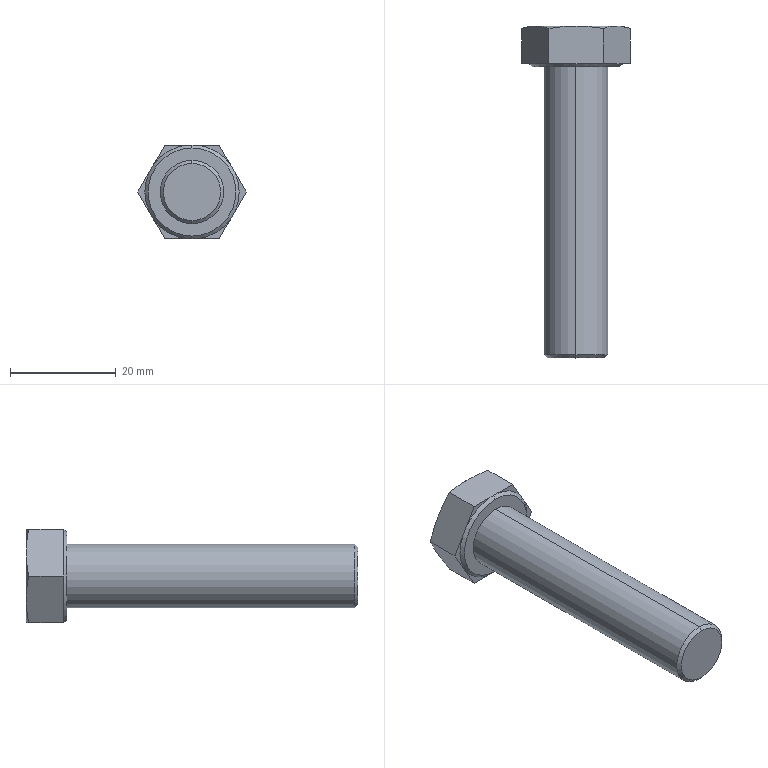Part | NX | features BREP 1 | 1 solid | 27 faces | box 20.473 x 62.68 x 17.73 mm | volume 8277 mm3 | plane 15 | cone 10 | cylinder 2 | commonest cylinder face diameters 12 x2
STEP:
#1=CARTESIAN_POINT('',(-41.42,-20.14,45.6));
#2=VERTEX_POINT('',#1);
#3=CARTESIAN_POINT('',(-41.42,-20.14,56.4));
#4=VERTEX_POINT('',#3);
#5=CARTESIAN_POINT('',(-41.42,-20.14,51.));
#6=DIRECTION('',(0.,-1.,0.));
#7=DIRECTION('',(0.,0.,-1.));
#8=AXIS2_PLACEMENT_3D('',#5,#6,#7);
#9=CIRCLE('',#8,5.4);
#10=EDGE_CURVE('',#2,#4,#9,.T.);
#11=ORIENTED_EDGE('',*,*,#10,.F.);
#12=CARTESIAN_POINT('',(-41.42,-19.54,45.));
#13=VERTEX_POINT('',#12);
#14=CARTESIAN_POINT('',(-41.42,-20.14,45.6));
#15=DIRECTION('',(0.,0.7071,-0.7071));
#16=VECTOR('',#15,1000.);
#17=LINE('',#14,#16);
#18=EDGE_CURVE('',#2,#13,#17,.T.);
#19=ORIENTED_EDGE('',*,*,#18,.T.);
#20=CARTESIAN_POINT('',(-41.42,-19.54,57.));
#21=VERTEX_POINT('',#20);
#22=CARTESIAN_POINT('',(-41.42,-19.54,51.));
#23=DIRECTION('',(0.,1.,0.));
#24=DIRECTION('',(0.,0.,-1.));
#25=AXIS2_PLACEMENT_3D('',#22,#23,#24);
#26=CIRCLE('',#25,6.);
#27=EDGE_CURVE('',#21,#13,#26,.T.);
#28=ORIENTED_EDGE('',*,*,#27,.F.);
#29=CARTESIAN_POINT('',(-41.42,-20.14,56.4));
#30=DIRECTION('',(0.,0.7071,0.7071));
#31=VECTOR('',#30,1000.);
#32=LINE('',#29,#31);
#33=EDGE_CURVE('',#4,#21,#32,.T.);
#34=ORIENTED_EDGE('',*,*,#33,.F.);
#35=EDGE_LOOP('',(#11,#19,#28,#34));
#36=FACE_BOUND('',#35,.T.);
#37=CARTESIAN_POINT('',(-41.42,-20.14,51.));
#38=DIRECTION('',(0.,1.,0.));
#39=DIRECTION('',(0.,0.,-1.));
#40=AXIS2_PLACEMENT_3D('',#37,#38,#39);
#41=CONICAL_SURFACE('',#40,5.4,0.7854);
#42=ADVANCED_FACE('',(#36),#41,.T.);
#43=ORIENTED_EDGE('',*,*,#27,.T.);
#44=CARTESIAN_POINT('',(-41.42,34.86,45.));
#45=VERTEX_POINT('',#44);
#46=CARTESIAN_POINT('',(-41.42,-20.14,45.));
#47=DIRECTION('',(0.,1.,0.));
#48=VECTOR('',#47,1000.);
#49=LINE('',#46,#48);
#50=EDGE_CURVE('',#13,#45,#49,.T.);
#51=ORIENTED_EDGE('',*,*,#50,.T.);
#52=CARTESIAN_POINT('',(-41.42,34.86,57.));
#53=VERTEX_POINT('',#52);
#54=CARTESIAN_POINT('',(-41.42,34.86,51.));
#55=DIRECTION('',(0.,-1.,0.));
#56=DIRECTION('',(0.,0.,-1.));
#57=AXIS2_PLACEMENT_3D('',#54,#55,#56);
#58=CIRCLE('',#57,6.);
#59=EDGE_CURVE('',#45,#53,#58,.T.);
#60=ORIENTED_EDGE('',*,*,#59,.T.);
#61=CARTESIAN_POINT('',(-41.42,-20.14,57.));
#62=DIRECTION('',(0.,1.,0.));
#63=VECTOR('',#62,1000.);
#64=LINE('',#61,#63);
#65=EDGE_CURVE('',#21,#53,#64,.T.);
#66=ORIENTED_EDGE('',*,*,#65,.F.);
#67=EDGE_LOOP('',(#43,#51,#60,#66));
#68=FACE_BOUND('',#67,.T.);
#69=CARTESIAN_POINT('',(-41.42,-20.14,51.));
#70=DIRECTION('',(0.,1.,0.));
#71=DIRECTION('',(0.,0.,-1.));
#72=AXIS2_PLACEMENT_3D('',#69,#70,#71);
#73=CYLINDRICAL_SURFACE('',#72,6.);
#74=ADVANCED_FACE('',(#68),#73,.T.);
#75=CARTESIAN_POINT('',(-41.42,34.86,59.315));
#76=VERTEX_POINT('',#75);
#77=CARTESIAN_POINT('',(-41.42,34.86,42.685));
#78=VERTEX_POINT('',#77);
#79=CARTESIAN_POINT('',(-41.42,34.86,51.));
#80=DIRECTION('',(0.,1.,0.));
#81=DIRECTION('',(0.,0.,1.));
#82=AXIS2_PLACEMENT_3D('',#79,#80,#81);
#83=CIRCLE('',#82,8.315);
#84=EDGE_CURVE('',#76,#78,#83,.T.);
#85=ORIENTED_EDGE('',*,*,#84,.T.);
#86=CARTESIAN_POINT('',(-41.42,35.41,42.135));
#87=VERTEX_POINT('',#86);
#88=CARTESIAN_POINT('',(-41.42,35.46,42.085));
#89=DIRECTION('',(0.,0.7071,-0.7071));
#90=VECTOR('',#89,1000.);
#91=LINE('',#88,#90);
#92=EDGE_CURVE('',#78,#87,#91,.T.);
#93=ORIENTED_EDGE('',*,*,#92,.T.);
#94=CARTESIAN_POINT('',(-40.477,35.46,42.135));
#95=VERTEX_POINT('',#94);
#96=CARTESIAN_POINT('',(-41.42,35.41,42.135));
#97=CARTESIAN_POINT('',(-41.106,35.41,42.135));
#98=CARTESIAN_POINT('',(-40.791,35.427,42.135));
#99=CARTESIAN_POINT('',(-40.477,35.46,42.135));
#100=B_SPLINE_CURVE_WITH_KNOTS('',3,(#96,#97,#98,#99),.UNSPECIFIED.,.F.,.F.,(4,4),(0.,1.),.PIECEWISE_BEZIER_KNOTS.);
#101=EDGE_CURVE('',#87,#95,#100,.T.);
#102=ORIENTED_EDGE('',*,*,#101,.T.);
#103=CARTESIAN_POINT('',(-34.214,35.46,45.751));
#104=VERTEX_POINT('',#103);
#105=CARTESIAN_POINT('',(-41.42,35.46,51.));
#106=DIRECTION('',(0.,1.,0.));
#107=DIRECTION('',(0.,0.,1.));
#108=AXIS2_PLACEMENT_3D('',#105,#106,#107);
#109=CIRCLE('',#108,8.915);
#110=EDGE_CURVE('',#104,#95,#109,.T.);
#111=ORIENTED_EDGE('',*,*,#110,.F.);
#112=CARTESIAN_POINT('',(-33.271,35.46,47.384));
#113=VERTEX_POINT('',#112);
#114=CARTESIAN_POINT('',(-34.214,35.46,45.751));
#115=CARTESIAN_POINT('',(-33.9,35.394,46.295));
#116=CARTESIAN_POINT('',(-33.586,35.394,46.84));
#117=CARTESIAN_POINT('',(-33.271,35.46,47.384));
#118=B_SPLINE_CURVE_WITH_KNOTS('',3,(#114,#115,#116,#117),.UNSPECIFIED.,.F.,.F.,(4,4),(0.,0.001886),.UNSPECIFIED.);
#119=EDGE_CURVE('',#104,#113,#118,.T.);
#120=ORIENTED_EDGE('',*,*,#119,.T.);
#121=CARTESIAN_POINT('',(-33.271,35.46,54.616));
#122=VERTEX_POINT('',#121);
#123=CARTESIAN_POINT('',(-41.42,35.46,51.));
#124=DIRECTION('',(0.,1.,0.));
#125=DIRECTION('',(0.,0.,1.));
#126=AXIS2_PLACEMENT_3D('',#123,#124,#125);
#127=CIRCLE('',#126,8.915);
#128=EDGE_CURVE('',#122,#113,#127,.T.);
#129=ORIENTED_EDGE('',*,*,#128,.F.);
#130=CARTESIAN_POINT('',(-34.214,35.46,56.249));
#131=VERTEX_POINT('',#130);
#132=CARTESIAN_POINT('',(-33.271,35.46,54.616));
#133=CARTESIAN_POINT('',(-33.586,35.394,55.16));
#134=CARTESIAN_POINT('',(-33.9,35.394,55.705));
#135=CARTESIAN_POINT('',(-34.214,35.46,56.249));
#136=B_SPLINE_CURVE_WITH_KNOTS('',3,(#132,#133,#134,#135),.UNSPECIFIED.,.F.,.F.,(4,4),(0.,0.001886),.UNSPECIFIED.);
#137=EDGE_CURVE('',#122,#131,#136,.T.);
#138=ORIENTED_EDGE('',*,*,#137,.T.);
#139=CARTESIAN_POINT('',(-40.477,35.46,59.865));
#140=VERTEX_POINT('',#139);
#141=CARTESIAN_POINT('',(-41.42,35.46,51.));
#142=DIRECTION('',(0.,1.,0.));
#143=DIRECTION('',(0.,0.,1.));
#144=AXIS2_PLACEMENT_3D('',#141,#142,#143);
#145=CIRCLE('',#144,8.915);
#146=EDGE_CURVE('',#140,#131,#145,.T.);
#147=ORIENTED_EDGE('',*,*,#146,.F.);
#148=CARTESIAN_POINT('',(-41.42,35.41,59.865));
#149=VERTEX_POINT('',#148);
#150=CARTESIAN_POINT('',(-40.477,35.46,59.865));
#151=CARTESIAN_POINT('',(-40.791,35.427,59.865));
#152=CARTESIAN_POINT('',(-41.106,35.41,59.865));
#153=CARTESIAN_POINT('',(-41.42,35.41,59.865));
#154=B_SPLINE_CURVE_WITH_KNOTS('',3,(#150,#151,#152,#153),.UNSPECIFIED.,.F.,.F.,(4,4),(0.,1.),.PIECEWISE_BEZIER_KNOTS.);
#155=EDGE_CURVE('',#140,#149,#154,.T.);
#156=ORIENTED_EDGE('',*,*,#155,.T.);
#157=CARTESIAN_POINT('',(-41.42,35.46,59.915));
#158=DIRECTION('',(0.,0.7071,0.7071));
#159=VECTOR('',#158,1000.);
#160=LINE('',#157,#159);
#161=EDGE_CURVE('',#76,#149,#160,.T.);
#162=ORIENTED_EDGE('',*,*,#161,.F.);
#163=EDGE_LOOP('',(#85,#93,#102,#111,#120,#129,#138,#147,#156,#162));
#164=FACE_BOUND('',#163,.T.);
#165=CARTESIAN_POINT('',(-41.42,35.46,51.));
#166=DIRECTION('',(0.,1.,0.));
#167=DIRECTION('',(0.,0.,-1.));
#168=AXIS2_PLACEMENT_3D('',#165,#166,#167);
#169=CONICAL_SURFACE('',#168,8.915,0.7854);
#170=ADVANCED_FACE('',(#164),#169,.T.);
#171=ORIENTED_EDGE('',*,*,#84,.F.);
#172=CARTESIAN_POINT('',(-41.42,34.86,51.));
#173=DIRECTION('',(0.,1.,0.));
#174=DIRECTION('',(0.,0.,1.));
#175=AXIS2_PLACEMENT_3D('',#172,#173,#174);
#176=CIRCLE('',#175,8.315);
#177=EDGE_CURVE('',#78,#76,#176,.T.);
#178=ORIENTED_EDGE('',*,*,#177,.F.);
#179=EDGE_LOOP('',(#171,#178));
#180=FACE_BOUND('',#179,.T.);
#181=CARTESIAN_POINT('',(-41.42,34.86,51.));
#182=DIRECTION('',(0.,-1.,0.));
#183=DIRECTION('',(0.,0.,-1.));
#184=AXIS2_PLACEMENT_3D('',#181,#182,#183);
#185=CIRCLE('',#184,6.);
#186=EDGE_CURVE('',#53,#45,#185,.T.);
#187=ORIENTED_EDGE('',*,*,#186,.F.);
#188=ORIENTED_EDGE('',*,*,#59,.F.);
#189=EDGE_LOOP('',(#187,#188));
#190=FACE_BOUND('',#189,.T.);
#191=CARTESIAN_POINT('',(-46.538,34.86,42.135));
#192=DIRECTION('',(0.,-1.,0.));
#193=DIRECTION('',(0.,0.,1.));
#194=AXIS2_PLACEMENT_3D('',#191,#192,#193);
#195=PLANE('',#194);
#196=ADVANCED_FACE('',(#180,#190),#195,.T.);
#197=CARTESIAN_POINT('',(-46.538,42.041,42.135));
#198=VERTEX_POINT('',#197);
#199=CARTESIAN_POINT('',(-49.097,42.54,46.568));
#200=VERTEX_POINT('',#199);
#201=CARTESIAN_POINT('',(-46.538,42.041,42.135));
#202=CARTESIAN_POINT('',(-47.384,42.349,43.601));
#203=CARTESIAN_POINT('',(-48.236,42.54,45.076));
#204=CARTESIAN_POINT('',(-49.097,42.54,46.568));
#205=B_SPLINE_CURVE_WITH_KNOTS('',3,(#201,#202,#203,#204),.UNSPECIFIED.,.F.,.F.,(4,4),(0.,0.005142),.UNSPECIFIED.);
#206=EDGE_CURVE('',#198,#200,#205,.T.);
#207=ORIENTED_EDGE('',*,*,#206,.F.);
#208=CARTESIAN_POINT('',(-46.538,35.46,42.135));
#209=VERTEX_POINT('',#208);
#210=CARTESIAN_POINT('',(-46.538,34.86,42.135));
#211=DIRECTION('',(0.,1.,0.));
#212=VECTOR('',#211,1000.);
#213=LINE('',#210,#212);
#214=EDGE_CURVE('',#209,#198,#213,.T.);
#215=ORIENTED_EDGE('',*,*,#214,.F.);
#216=CARTESIAN_POINT('',(-48.626,35.46,45.751));
#217=VERTEX_POINT('',#216);
#218=CARTESIAN_POINT('',(-51.656,35.46,51.));
#219=DIRECTION('',(0.5,0.,-0.866));
#220=VECTOR('',#219,1000.);
#221=LINE('',#218,#220);
#222=EDGE_CURVE('',#217,#209,#221,.T.);
#223=ORIENTED_EDGE('',*,*,#222,.F.);
#224=CARTESIAN_POINT('',(-49.569,35.46,47.384));
#225=VERTEX_POINT('',#224);
#226=CARTESIAN_POINT('',(-49.569,35.46,47.384));
#227=CARTESIAN_POINT('',(-49.255,35.394,46.84));
#228=CARTESIAN_POINT('',(-48.94,35.394,46.295));
#229=CARTESIAN_POINT('',(-48.626,35.46,45.751));
#230=B_SPLINE_CURVE_WITH_KNOTS('',3,(#226,#227,#228,#229),.UNSPECIFIED.,.F.,.F.,(4,4),(0.,0.001886),.UNSPECIFIED.);
#231=EDGE_CURVE('',#225,#217,#230,.T.);
#232=ORIENTED_EDGE('',*,*,#231,.F.);
#233=CARTESIAN_POINT('',(-51.656,35.46,51.));
#234=VERTEX_POINT('',#233);
#235=CARTESIAN_POINT('',(-51.656,35.46,51.));
#236=DIRECTION('',(0.5,0.,-0.866));
#237=VECTOR('',#236,1000.);
#238=LINE('',#235,#237);
#239=EDGE_CURVE('',#234,#225,#238,.T.);
#240=ORIENTED_EDGE('',*,*,#239,.F.);
#241=CARTESIAN_POINT('',(-51.656,42.041,51.));
#242=VERTEX_POINT('',#241);
#243=CARTESIAN_POINT('',(-51.656,34.86,51.));
#244=DIRECTION('',(0.,1.,0.));
#245=VECTOR('',#244,1000.);
#246=LINE('',#243,#245);
#247=EDGE_CURVE('',#234,#242,#246,.T.);
#248=ORIENTED_EDGE('',*,*,#247,.T.);
#249=CARTESIAN_POINT('',(-49.097,42.54,46.568));
#250=CARTESIAN_POINT('',(-49.959,42.54,48.059));
#251=CARTESIAN_POINT('',(-50.81,42.349,49.534));
#252=CARTESIAN_POINT('',(-51.656,42.041,51.));
#253=B_SPLINE_CURVE_WITH_KNOTS('',3,(#249,#250,#251,#252),.UNSPECIFIED.,.F.,.F.,(4,4),(0.,0.005142),.UNSPECIFIED.);
#254=EDGE_CURVE('',#200,#242,#253,.T.);
#255=ORIENTED_EDGE('',*,*,#254,.F.);
#256=EDGE_LOOP('',(#207,#215,#223,#232,#240,#248,#255));
#257=FACE_BOUND('',#256,.T.);
#258=CARTESIAN_POINT('',(-51.656,34.86,51.));
#259=DIRECTION('',(0.866,0.,0.5));
#260=DIRECTION('',(0.5,0.,-0.866));
#261=AXIS2_PLACEMENT_3D('',#258,#259,#260);
#262=PLANE('',#261);
#263=ADVANCED_FACE('',(#257),#262,.F.);
#264=CARTESIAN_POINT('',(-36.302,42.041,42.135));
#265=VERTEX_POINT('',#264);
#266=CARTESIAN_POINT('',(-41.42,42.54,42.135));
#267=VERTEX_POINT('',#266);
#268=CARTESIAN_POINT('',(-36.302,42.041,42.135));
#269=CARTESIAN_POINT('',(-37.994,42.349,42.135));
#270=CARTESIAN_POINT('',(-39.698,42.54,42.135));
#271=CARTESIAN_POINT('',(-41.42,42.54,42.135));
#272=B_SPLINE_CURVE_WITH_KNOTS('',3,(#268,#269,#270,#271),.UNSPECIFIED.,.F.,.F.,(4,4),(0.,0.005142),.UNSPECIFIED.);
#273=EDGE_CURVE('',#265,#267,#272,.T.);
#274=ORIENTED_EDGE('',*,*,#273,.F.);
#275=CARTESIAN_POINT('',(-36.302,35.46,42.135));
#276=VERTEX_POINT('',#275);
#277=CARTESIAN_POINT('',(-36.302,34.86,42.135));
#278=DIRECTION('',(0.,1.,0.));
#279=VECTOR('',#278,1000.);
#280=LINE('',#277,#279);
#281=EDGE_CURVE('',#276,#265,#280,.T.);
#282=ORIENTED_EDGE('',*,*,#281,.F.);
#283=CARTESIAN_POINT('',(-46.538,35.46,42.135));
#284=DIRECTION('',(1.,0.,0.));
#285=VECTOR('',#284,1000.);
#286=LINE('',#283,#285);
#287=EDGE_CURVE('',#95,#276,#286,.T.);
#288=ORIENTED_EDGE('',*,*,#287,.F.);
#289=ORIENTED_EDGE('',*,*,#101,.F.);
#290=CARTESIAN_POINT('',(-42.363,35.46,42.135));
#291=VERTEX_POINT('',#290);
#292=CARTESIAN_POINT('',(-42.363,35.46,42.135));
#293=CARTESIAN_POINT('',(-42.048,35.427,42.135));
#294=CARTESIAN_POINT('',(-41.734,35.41,42.135));
#295=CARTESIAN_POINT('',(-41.42,35.41,42.135));
#296=B_SPLINE_CURVE_WITH_KNOTS('',3,(#292,#293,#294,#295),.UNSPECIFIED.,.F.,.F.,(4,4),(0.,1.),.PIECEWISE_BEZIER_KNOTS.);
#297=EDGE_CURVE('',#291,#87,#296,.T.);
#298=ORIENTED_EDGE('',*,*,#297,.F.);
#299=CARTESIAN_POINT('',(-46.538,35.46,42.135));
#300=DIRECTION('',(1.,0.,0.));
#301=VECTOR('',#300,1000.);
#302=LINE('',#299,#301);
#303=EDGE_CURVE('',#209,#291,#302,.T.);
#304=ORIENTED_EDGE('',*,*,#303,.F.);
#305=ORIENTED_EDGE('',*,*,#214,.T.);
#306=CARTESIAN_POINT('',(-41.42,42.54,42.135));
#307=CARTESIAN_POINT('',(-43.142,42.54,42.135));
#308=CARTESIAN_POINT('',(-44.846,42.349,42.135));
#309=CARTESIAN_POINT('',(-46.538,42.041,42.135));
#310=B_SPLINE_CURVE_WITH_KNOTS('',3,(#306,#307,#308,#309),.UNSPECIFIED.,.F.,.F.,(4,4),(0.,0.005142),.UNSPECIFIED.);
#311=EDGE_CURVE('',#267,#198,#310,.T.);
#312=ORIENTED_EDGE('',*,*,#311,.F.);
#313=EDGE_LOOP('',(#274,#282,#288,#289,#298,#304,#305,#312));
#314=FACE_BOUND('',#313,.T.);
#315=CARTESIAN_POINT('',(-46.538,34.86,42.135));
#316=DIRECTION('',(0.,0.,1.));
#317=DIRECTION('',(0.,1.,0.));
#318=AXIS2_PLACEMENT_3D('',#315,#316,#317);
#319=PLANE('',#318);
#320=ADVANCED_FACE('',(#314),#319,.F.);
#321=CARTESIAN_POINT('',(-31.184,42.041,51.));
#322=VERTEX_POINT('',#321);
#323=CARTESIAN_POINT('',(-33.743,42.54,46.568));
#324=VERTEX_POINT('',#323);
#325=CARTESIAN_POINT('',(-31.184,42.041,51.));
#326=CARTESIAN_POINT('',(-32.03,42.349,49.534));
#327=CARTESIAN_POINT('',(-32.882,42.54,48.059));
#328=CARTESIAN_POINT('',(-33.743,42.54,46.568));
#329=B_SPLINE_CURVE_WITH_KNOTS('',3,(#325,#326,#327,#328),.UNSPECIFIED.,.F.,.F.,(4,4),(0.,0.005142),.UNSPECIFIED.);
#330=EDGE_CURVE('',#322,#324,#329,.T.);
#331=ORIENTED_EDGE('',*,*,#330,.F.);
#332=CARTESIAN_POINT('',(-31.184,35.46,51.));
#333=VERTEX_POINT('',#332);
#334=CARTESIAN_POINT('',(-31.184,34.86,51.));
#335=DIRECTION('',(0.,1.,0.));
#336=VECTOR('',#335,1000.);
#337=LINE('',#334,#336);
#338=EDGE_CURVE('',#333,#322,#337,.T.);
#339=ORIENTED_EDGE('',*,*,#338,.F.);
#340=CARTESIAN_POINT('',(-36.302,35.46,42.135));
#341=DIRECTION('',(0.5,0.,0.866));
#342=VECTOR('',#341,1000.);
#343=LINE('',#340,#342);
#344=EDGE_CURVE('',#113,#333,#343,.T.);
#345=ORIENTED_EDGE('',*,*,#344,.F.);
#346=ORIENTED_EDGE('',*,*,#119,.F.);
#347=CARTESIAN_POINT('',(-36.302,35.46,42.135));
#348=DIRECTION('',(0.5,0.,0.866));
#349=VECTOR('',#348,1000.);
#350=LINE('',#347,#349);
#351=EDGE_CURVE('',#276,#104,#350,.T.);
#352=ORIENTED_EDGE('',*,*,#351,.F.);
#353=ORIENTED_EDGE('',*,*,#281,.T.);
#354=CARTESIAN_POINT('',(-33.743,42.54,46.568));
#355=CARTESIAN_POINT('',(-34.604,42.54,45.076));
#356=CARTESIAN_POINT('',(-35.456,42.349,43.601));
#357=CARTESIAN_POINT('',(-36.302,42.041,42.135));
#358=B_SPLINE_CURVE_WITH_KNOTS('',3,(#354,#355,#356,#357),.UNSPECIFIED.,.F.,.F.,(4,4),(0.,0.005142),.UNSPECIFIED.);
#359=EDGE_CURVE('',#324,#265,#358,.T.);
#360=ORIENTED_EDGE('',*,*,#359,.F.);
#361=EDGE_LOOP('',(#331,#339,#345,#346,#352,#353,#360));
#362=FACE_BOUND('',#361,.T.);
#363=CARTESIAN_POINT('',(-36.302,34.86,42.135));
#364=DIRECTION('',(-0.866,0.,0.5));
#365=DIRECTION('',(0.5,0.,0.866));
#366=AXIS2_PLACEMENT_3D('',#363,#364,#365);
#367=PLANE('',#366);
#368=ADVANCED_FACE('',(#362),#367,.F.);
#369=CARTESIAN_POINT('',(-36.302,42.041,59.865));
#370=VERTEX_POINT('',#369);
#371=CARTESIAN_POINT('',(-33.743,42.54,55.432));
#372=VERTEX_POINT('',#371);
#373=CARTESIAN_POINT('',(-36.302,42.041,59.865));
#374=CARTESIAN_POINT('',(-35.456,42.349,58.399));
#375=CARTESIAN_POINT('',(-34.604,42.54,56.924));
#376=CARTESIAN_POINT('',(-33.743,42.54,55.432));
#377=B_SPLINE_CURVE_WITH_KNOTS('',3,(#373,#374,#375,#376),.UNSPECIFIED.,.F.,.F.,(4,4),(0.,0.005142),.UNSPECIFIED.);
#378=EDGE_CURVE('',#370,#372,#377,.T.);
#379=ORIENTED_EDGE('',*,*,#378,.F.);
#380=CARTESIAN_POINT('',(-36.302,35.46,59.865));
#381=VERTEX_POINT('',#380);
#382=CARTESIAN_POINT('',(-36.302,34.86,59.865));
#383=DIRECTION('',(0.,1.,0.));
#384=VECTOR('',#383,1000.);
#385=LINE('',#382,#384);
#386=EDGE_CURVE('',#381,#370,#385,.T.);
#387=ORIENTED_EDGE('',*,*,#386,.F.);
#388=CARTESIAN_POINT('',(-31.184,35.46,51.));
#389=DIRECTION('',(-0.5,0.,0.866));
#390=VECTOR('',#389,1000.);
#391=LINE('',#388,#390);
#392=EDGE_CURVE('',#131,#381,#391,.T.);
#393=ORIENTED_EDGE('',*,*,#392,.F.);
#394=ORIENTED_EDGE('',*,*,#137,.F.);
#395=CARTESIAN_POINT('',(-31.184,35.46,51.));
#396=DIRECTION('',(-0.5,0.,0.866));
#397=VECTOR('',#396,1000.);
#398=LINE('',#395,#397);
#399=EDGE_CURVE('',#333,#122,#398,.T.);
#400=ORIENTED_EDGE('',*,*,#399,.F.);
#401=ORIENTED_EDGE('',*,*,#338,.T.);
#402=CARTESIAN_POINT('',(-33.743,42.54,55.432));
#403=CARTESIAN_POINT('',(-32.882,42.54,53.941));
#404=CARTESIAN_POINT('',(-32.03,42.349,52.466));
#405=CARTESIAN_POINT('',(-31.184,42.041,51.));
#406=B_SPLINE_CURVE_WITH_KNOTS('',3,(#402,#403,#404,#405),.UNSPECIFIED.,.F.,.F.,(4,4),(0.,0.005142),.UNSPECIFIED.);
#407=EDGE_CURVE('',#372,#322,#406,.T.);
#408=ORIENTED_EDGE('',*,*,#407,.F.);
#409=EDGE_LOOP('',(#379,#387,#393,#394,#400,#401,#408));
#410=FACE_BOUND('',#409,.T.);
#411=CARTESIAN_POINT('',(-31.184,34.86,51.));
#412=DIRECTION('',(-0.866,0.,-0.5));
#413=DIRECTION('',(-0.5,0.,0.866));
#414=AXIS2_PLACEMENT_3D('',#411,#412,#413);
#415=PLANE('',#414);
#416=ADVANCED_FACE('',(#410),#415,.F.);
#417=CARTESIAN_POINT('',(-46.538,42.041,59.865));
#418=VERTEX_POINT('',#417);
#419=CARTESIAN_POINT('',(-41.42,42.54,59.865));
#420=VERTEX_POINT('',#419);
#421=CARTESIAN_POINT('',(-46.538,42.041,59.865));
#422=CARTESIAN_POINT('',(-44.846,42.349,59.865));
#423=CARTESIAN_POINT('',(-43.142,42.54,59.865));
#424=CARTESIAN_POINT('',(-41.42,42.54,59.865));
#425=B_SPLINE_CURVE_WITH_KNOTS('',3,(#421,#422,#423,#424),.UNSPECIFIED.,.F.,.F.,(4,4),(0.,0.005142),.UNSPECIFIED.);
#426=EDGE_CURVE('',#418,#420,#425,.T.);
#427=ORIENTED_EDGE('',*,*,#426,.F.);
#428=CARTESIAN_POINT('',(-46.538,35.46,59.865));
#429=VERTEX_POINT('',#428);
#430=CARTESIAN_POINT('',(-46.538,34.86,59.865));
#431=DIRECTION('',(0.,1.,0.));
#432=VECTOR('',#431,1000.);
#433=LINE('',#430,#432);
#434=EDGE_CURVE('',#429,#418,#433,.T.);
#435=ORIENTED_EDGE('',*,*,#434,.F.);
#436=CARTESIAN_POINT('',(-42.363,35.46,59.865));
#437=VERTEX_POINT('',#436);
#438=CARTESIAN_POINT('',(-36.302,35.46,59.865));
#439=DIRECTION('',(-1.,0.,0.));
#440=VECTOR('',#439,1000.);
#441=LINE('',#438,#440);
#442=EDGE_CURVE('',#437,#429,#441,.T.);
#443=ORIENTED_EDGE('',*,*,#442,.F.);
#444=CARTESIAN_POINT('',(-41.42,35.41,59.865));
#445=CARTESIAN_POINT('',(-41.734,35.41,59.865));
#446=CARTESIAN_POINT('',(-42.048,35.427,59.865));
#447=CARTESIAN_POINT('',(-42.363,35.46,59.865));
#448=B_SPLINE_CURVE_WITH_KNOTS('',3,(#444,#445,#446,#447),.UNSPECIFIED.,.F.,.F.,(4,4),(0.,1.),.PIECEWISE_BEZIER_KNOTS.);
#449=EDGE_CURVE('',#149,#437,#448,.T.);
#450=ORIENTED_EDGE('',*,*,#449,.F.);
#451=ORIENTED_EDGE('',*,*,#155,.F.);
#452=CARTESIAN_POINT('',(-36.302,35.46,59.865));
#453=DIRECTION('',(-1.,0.,0.));
#454=VECTOR('',#453,1000.);
#455=LINE('',#452,#454);
#456=EDGE_CURVE('',#381,#140,#455,.T.);
#457=ORIENTED_EDGE('',*,*,#456,.F.);
#458=ORIENTED_EDGE('',*,*,#386,.T.);
#459=CARTESIAN_POINT('',(-41.42,42.54,59.865));
#460=CARTESIAN_POINT('',(-39.698,42.54,59.865));
#461=CARTESIAN_POINT('',(-37.994,42.349,59.865));
#462=CARTESIAN_POINT('',(-36.302,42.041,59.865));
#463=B_SPLINE_CURVE_WITH_KNOTS('',3,(#459,#460,#461,#462),.UNSPECIFIED.,.F.,.F.,(4,4),(0.,0.005142),.UNSPECIFIED.);
#464=EDGE_CURVE('',#420,#370,#463,.T.);
#465=ORIENTED_EDGE('',*,*,#464,.F.);
#466=EDGE_LOOP('',(#427,#435,#443,#450,#451,#457,#458,#465));
#467=FACE_BOUND('',#466,.T.);
#468=CARTESIAN_POINT('',(-36.302,34.86,59.865));
#469=DIRECTION('',(0.,0.,-1.));
#470=DIRECTION('',(0.,-1.,0.));
#471=AXIS2_PLACEMENT_3D('',#468,#469,#470);
#472=PLANE('',#471);
#473=ADVANCED_FACE('',(#467),#472,.F.);
#474=CARTESIAN_POINT('',(-49.097,42.54,55.432));
#475=VERTEX_POINT('',#474);
#476=CARTESIAN_POINT('',(-51.656,42.041,51.));
#477=CARTESIAN_POINT('',(-50.81,42.349,52.466));
#478=CARTESIAN_POINT('',(-49.959,42.54,53.941));
#479=CARTESIAN_POINT('',(-49.097,42.54,55.432));
#480=B_SPLINE_CURVE_WITH_KNOTS('',3,(#476,#477,#478,#479),.UNSPECIFIED.,.F.,.F.,(4,4),(0.,0.005142),.UNSPECIFIED.);
#481=EDGE_CURVE('',#242,#475,#480,.T.);
#482=ORIENTED_EDGE('',*,*,#481,.F.);
#483=ORIENTED_EDGE('',*,*,#247,.F.);
#484=CARTESIAN_POINT('',(-49.569,35.46,54.616));
#485=VERTEX_POINT('',#484);
#486=CARTESIAN_POINT('',(-46.538,35.46,59.865));
#487=DIRECTION('',(-0.5,0.,-0.866));
#488=VECTOR('',#487,1000.);
#489=LINE('',#486,#488);
#490=EDGE_CURVE('',#485,#234,#489,.T.);
#491=ORIENTED_EDGE('',*,*,#490,.F.);
#492=CARTESIAN_POINT('',(-48.626,35.46,56.249));
#493=VERTEX_POINT('',#492);
#494=CARTESIAN_POINT('',(-48.626,35.46,56.249));
#495=CARTESIAN_POINT('',(-48.94,35.394,55.705));
#496=CARTESIAN_POINT('',(-49.255,35.394,55.16));
#497=CARTESIAN_POINT('',(-49.569,35.46,54.616));
#498=B_SPLINE_CURVE_WITH_KNOTS('',3,(#494,#495,#496,#497),.UNSPECIFIED.,.F.,.F.,(4,4),(0.,0.001886),.UNSPECIFIED.);
#499=EDGE_CURVE('',#493,#485,#498,.T.);
#500=ORIENTED_EDGE('',*,*,#499,.F.);
#501=CARTESIAN_POINT('',(-46.538,35.46,59.865));
#502=DIRECTION('',(-0.5,0.,-0.866));
#503=VECTOR('',#502,1000.);
#504=LINE('',#501,#503);
#505=EDGE_CURVE('',#429,#493,#504,.T.);
#506=ORIENTED_EDGE('',*,*,#505,.F.);
#507=ORIENTED_EDGE('',*,*,#434,.T.);
#508=CARTESIAN_POINT('',(-49.097,42.54,55.432));
#509=CARTESIAN_POINT('',(-48.236,42.54,56.924));
#510=CARTESIAN_POINT('',(-47.384,42.349,58.399));
#511=CARTESIAN_POINT('',(-46.538,42.041,59.865));
#512=B_SPLINE_CURVE_WITH_KNOTS('',3,(#508,#509,#510,#511),.UNSPECIFIED.,.F.,.F.,(4,4),(0.,0.005142),.UNSPECIFIED.);
#513=EDGE_CURVE('',#475,#418,#512,.T.);
#514=ORIENTED_EDGE('',*,*,#513,.F.);
#515=EDGE_LOOP('',(#482,#483,#491,#500,#506,#507,#514));
#516=FACE_BOUND('',#515,.T.);
#517=CARTESIAN_POINT('',(-46.538,34.86,59.865));
#518=DIRECTION('',(0.866,0.,-0.5));
#519=DIRECTION('',(-0.5,0.,-0.866));
#520=AXIS2_PLACEMENT_3D('',#517,#518,#519);
#521=PLANE('',#520);
#522=ADVANCED_FACE('',(#516),#521,.F.);
#523=ORIENTED_EDGE('',*,*,#222,.T.);
#524=ORIENTED_EDGE('',*,*,#303,.T.);
#525=CARTESIAN_POINT('',(-41.42,35.46,51.));
#526=DIRECTION('',(0.,1.,0.));
#527=DIRECTION('',(0.,0.,1.));
#528=AXIS2_PLACEMENT_3D('',#525,#526,#527);
#529=CIRCLE('',#528,8.915);
#530=EDGE_CURVE('',#291,#217,#529,.T.);
#531=ORIENTED_EDGE('',*,*,#530,.T.);
#532=EDGE_LOOP('',(#523,#524,#531));
#533=FACE_BOUND('',#532,.T.);
#534=CARTESIAN_POINT('',(-32.505,35.46,51.));
#535=DIRECTION('',(0.,-1.,0.));
#536=DIRECTION('',(0.,0.,1.));
#537=AXIS2_PLACEMENT_3D('',#534,#535,#536);
#538=PLANE('',#537);
#539=ADVANCED_FACE('',(#533),#538,.T.);
#540=ORIENTED_EDGE('',*,*,#287,.T.);
#541=ORIENTED_EDGE('',*,*,#351,.T.);
#542=ORIENTED_EDGE('',*,*,#110,.T.);
#543=EDGE_LOOP('',(#540,#541,#542));
#544=FACE_BOUND('',#543,.T.);
#545=CARTESIAN_POINT('',(-32.505,35.46,51.));
#546=DIRECTION('',(0.,-1.,0.));
#547=DIRECTION('',(0.,0.,1.));
#548=AXIS2_PLACEMENT_3D('',#545,#546,#547);
#549=PLANE('',#548);
#550=ADVANCED_FACE('',(#544),#549,.T.);
#551=ORIENTED_EDGE('',*,*,#344,.T.);
#552=ORIENTED_EDGE('',*,*,#399,.T.);
#553=ORIENTED_EDGE('',*,*,#128,.T.);
#554=EDGE_LOOP('',(#551,#552,#553));
#555=FACE_BOUND('',#554,.T.);
#556=CARTESIAN_POINT('',(-32.505,35.46,51.));
#557=DIRECTION('',(0.,-1.,0.));
#558=DIRECTION('',(0.,0.,1.));
#559=AXIS2_PLACEMENT_3D('',#556,#557,#558);
#560=PLANE('',#559);
#561=ADVANCED_FACE('',(#555),#560,.T.);
#562=ORIENTED_EDGE('',*,*,#392,.T.);
#563=ORIENTED_EDGE('',*,*,#456,.T.);
#564=ORIENTED_EDGE('',*,*,#146,.T.);
#565=EDGE_LOOP('',(#562,#563,#564));
#566=FACE_BOUND('',#565,.T.);
#567=CARTESIAN_POINT('',(-32.505,35.46,51.));
#568=DIRECTION('',(0.,-1.,0.));
#569=DIRECTION('',(0.,0.,1.));
#570=AXIS2_PLACEMENT_3D('',#567,#568,#569);
#571=PLANE('',#570);
#572=ADVANCED_FACE('',(#566),#571,.T.);
#573=ORIENTED_EDGE('',*,*,#442,.T.);
#574=ORIENTED_EDGE('',*,*,#505,.T.);
#575=CARTESIAN_POINT('',(-41.42,35.46,51.));
#576=DIRECTION('',(0.,1.,0.));
#577=DIRECTION('',(0.,0.,1.));
#578=AXIS2_PLACEMENT_3D('',#575,#576,#577);
#579=CIRCLE('',#578,8.915);
#580=EDGE_CURVE('',#493,#437,#579,.T.);
#581=ORIENTED_EDGE('',*,*,#580,.T.);
#582=EDGE_LOOP('',(#573,#574,#581));
#583=FACE_BOUND('',#582,.T.);
#584=CARTESIAN_POINT('',(-32.505,35.46,51.));
#585=DIRECTION('',(0.,-1.,0.));
#586=DIRECTION('',(0.,0.,1.));
#587=AXIS2_PLACEMENT_3D('',#584,#585,#586);
#588=PLANE('',#587);
#589=ADVANCED_FACE('',(#583),#588,.T.);
#590=ORIENTED_EDGE('',*,*,#239,.T.);
#591=CARTESIAN_POINT('',(-41.42,35.46,51.));
#592=DIRECTION('',(0.,1.,0.));
#593=DIRECTION('',(0.,0.,1.));
#594=AXIS2_PLACEMENT_3D('',#591,#592,#593);
#595=CIRCLE('',#594,8.915);
#596=EDGE_CURVE('',#225,#485,#595,.T.);
#597=ORIENTED_EDGE('',*,*,#596,.T.);
#598=ORIENTED_EDGE('',*,*,#490,.T.);
#599=EDGE_LOOP('',(#590,#597,#598));
#600=FACE_BOUND('',#599,.T.);
#601=CARTESIAN_POINT('',(-32.505,35.46,51.));
#602=DIRECTION('',(0.,-1.,0.));
#603=DIRECTION('',(0.,0.,1.));
#604=AXIS2_PLACEMENT_3D('',#601,#602,#603);
#605=PLANE('',#604);
#606=ADVANCED_FACE('',(#600),#605,.T.);
#607=ORIENTED_EDGE('',*,*,#92,.F.);
#608=ORIENTED_EDGE('',*,*,#177,.T.);
#609=ORIENTED_EDGE('',*,*,#161,.T.);
#610=ORIENTED_EDGE('',*,*,#449,.T.);
#611=ORIENTED_EDGE('',*,*,#580,.F.);
#612=ORIENTED_EDGE('',*,*,#499,.T.);
#613=ORIENTED_EDGE('',*,*,#596,.F.);
#614=ORIENTED_EDGE('',*,*,#231,.T.);
#615=ORIENTED_EDGE('',*,*,#530,.F.);
#616=ORIENTED_EDGE('',*,*,#297,.T.);
#617=EDGE_LOOP('',(#607,#608,#609,#610,#611,#612,#613,#614,#615,#616));
#618=FACE_BOUND('',#617,.T.);
#619=CARTESIAN_POINT('',(-41.42,35.46,51.));
#620=DIRECTION('',(0.,1.,0.));
#621=DIRECTION('',(0.,0.,-1.));
#622=AXIS2_PLACEMENT_3D('',#619,#620,#621);
#623=CONICAL_SURFACE('',#622,8.915,0.7854);
#624=ADVANCED_FACE('',(#618),#623,.T.);
#625=ORIENTED_EDGE('',*,*,#311,.T.);
#626=ORIENTED_EDGE('',*,*,#206,.T.);
#627=CARTESIAN_POINT('',(-41.42,42.54,51.));
#628=DIRECTION('',(0.,-1.,0.));
#629=DIRECTION('',(0.,0.,-1.));
#630=AXIS2_PLACEMENT_3D('',#627,#628,#629);
#631=CIRCLE('',#630,8.865);
#632=EDGE_CURVE('',#200,#267,#631,.T.);
#633=ORIENTED_EDGE('',*,*,#632,.T.);
#634=EDGE_LOOP('',(#625,#626,#633));
#635=FACE_BOUND('',#634,.T.);
#636=CARTESIAN_POINT('',(-41.42,42.54,51.));
#637=DIRECTION('',(0.,-1.,0.));
#638=DIRECTION('',(0.,0.,1.));
#639=AXIS2_PLACEMENT_3D('',#636,#637,#638);
#640=CONICAL_SURFACE('',#639,8.865,1.222);
#641=ADVANCED_FACE('',(#635),#640,.T.);
#642=ORIENTED_EDGE('',*,*,#254,.T.);
#643=ORIENTED_EDGE('',*,*,#481,.T.);
#644=CARTESIAN_POINT('',(-41.42,42.54,51.));
#645=DIRECTION('',(0.,-1.,0.));
#646=DIRECTION('',(0.,0.,-1.));
#647=AXIS2_PLACEMENT_3D('',#644,#645,#646);
#648=CIRCLE('',#647,8.865);
#649=EDGE_CURVE('',#475,#200,#648,.T.);
#650=ORIENTED_EDGE('',*,*,#649,.T.);
#651=EDGE_LOOP('',(#642,#643,#650));
#652=FACE_BOUND('',#651,.T.);
#653=CARTESIAN_POINT('',(-41.42,42.54,51.));
#654=DIRECTION('',(0.,-1.,0.));
#655=DIRECTION('',(0.,0.,1.));
#656=AXIS2_PLACEMENT_3D('',#653,#654,#655);
#657=CONICAL_SURFACE('',#656,8.865,1.222);
#658=ADVANCED_FACE('',(#652),#657,.T.);
#659=ORIENTED_EDGE('',*,*,#426,.T.);
#660=CARTESIAN_POINT('',(-41.42,42.54,51.));
#661=DIRECTION('',(0.,-1.,0.));
#662=DIRECTION('',(0.,0.,-1.));
#663=AXIS2_PLACEMENT_3D('',#660,#661,#662);
#664=CIRCLE('',#663,8.865);
#665=EDGE_CURVE('',#420,#475,#664,.T.);
#666=ORIENTED_EDGE('',*,*,#665,.T.);
#667=ORIENTED_EDGE('',*,*,#513,.T.);
#668=EDGE_LOOP('',(#659,#666,#667));
#669=FACE_BOUND('',#668,.T.);
#670=CARTESIAN_POINT('',(-41.42,42.54,51.));
#671=DIRECTION('',(0.,-1.,0.));
#672=DIRECTION('',(0.,0.,1.));
#673=AXIS2_PLACEMENT_3D('',#670,#671,#672);
#674=CONICAL_SURFACE('',#673,8.865,1.222);
#675=ADVANCED_FACE('',(#669),#674,.T.);
#676=ORIENTED_EDGE('',*,*,#378,.T.);
#677=CARTESIAN_POINT('',(-41.42,42.54,51.));
#678=DIRECTION('',(0.,1.,0.));
#679=DIRECTION('',(0.,0.,1.));
#680=AXIS2_PLACEMENT_3D('',#677,#678,#679);
#681=CIRCLE('',#680,8.865);
#682=EDGE_CURVE('',#420,#372,#681,.T.);
#683=ORIENTED_EDGE('',*,*,#682,.F.);
#684=ORIENTED_EDGE('',*,*,#464,.T.);
#685=EDGE_LOOP('',(#676,#683,#684));
#686=FACE_BOUND('',#685,.T.);
#687=CARTESIAN_POINT('',(-41.42,42.54,51.));
#688=DIRECTION('',(0.,-1.,0.));
#689=DIRECTION('',(0.,0.,1.));
#690=AXIS2_PLACEMENT_3D('',#687,#688,#689);
#691=CONICAL_SURFACE('',#690,8.865,1.222);
#692=ADVANCED_FACE('',(#686),#691,.T.);
#693=ORIENTED_EDGE('',*,*,#330,.T.);
#694=CARTESIAN_POINT('',(-41.42,42.54,51.));
#695=DIRECTION('',(0.,-1.,0.));
#696=DIRECTION('',(0.,0.,-1.));
#697=AXIS2_PLACEMENT_3D('',#694,#695,#696);
#698=CIRCLE('',#697,8.865);
#699=EDGE_CURVE('',#324,#372,#698,.T.);
#700=ORIENTED_EDGE('',*,*,#699,.T.);
#701=ORIENTED_EDGE('',*,*,#407,.T.);
#702=EDGE_LOOP('',(#693,#700,#701));
#703=FACE_BOUND('',#702,.T.);
#704=CARTESIAN_POINT('',(-41.42,42.54,51.));
#705=DIRECTION('',(0.,-1.,0.));
#706=DIRECTION('',(0.,0.,1.));
#707=AXIS2_PLACEMENT_3D('',#704,#705,#706);
#708=CONICAL_SURFACE('',#707,8.865,1.222);
#709=ADVANCED_FACE('',(#703),#708,.T.);
#710=ORIENTED_EDGE('',*,*,#359,.T.);
#711=ORIENTED_EDGE('',*,*,#273,.T.);
#712=CARTESIAN_POINT('',(-41.42,42.54,51.));
#713=DIRECTION('',(0.,-1.,0.));
#714=DIRECTION('',(0.,0.,-1.));
#715=AXIS2_PLACEMENT_3D('',#712,#713,#714);
#716=CIRCLE('',#715,8.865);
#717=EDGE_CURVE('',#267,#324,#716,.T.);
#718=ORIENTED_EDGE('',*,*,#717,.T.);
#719=EDGE_LOOP('',(#710,#711,#718));
#720=FACE_BOUND('',#719,.T.);
#721=CARTESIAN_POINT('',(-41.42,42.54,51.));
#722=DIRECTION('',(0.,-1.,0.));
#723=DIRECTION('',(0.,0.,1.));
#724=AXIS2_PLACEMENT_3D('',#721,#722,#723);
#725=CONICAL_SURFACE('',#724,8.865,1.222);
#726=ADVANCED_FACE('',(#720),#725,.T.);
#727=ORIENTED_EDGE('',*,*,#717,.F.);
#728=ORIENTED_EDGE('',*,*,#632,.F.);
#729=ORIENTED_EDGE('',*,*,#649,.F.);
#730=ORIENTED_EDGE('',*,*,#665,.F.);
#731=ORIENTED_EDGE('',*,*,#682,.T.);
#732=ORIENTED_EDGE('',*,*,#699,.F.);
#733=EDGE_LOOP('',(#727,#728,#729,#730,#731,#732));
#734=FACE_BOUND('',#733,.T.);
#735=CARTESIAN_POINT('',(-46.538,42.54,42.135));
#736=DIRECTION('',(0.,-1.,0.));
#737=DIRECTION('',(0.,0.,1.));
#738=AXIS2_PLACEMENT_3D('',#735,#736,#737);
#739=PLANE('',#738);
#740=ADVANCED_FACE('',(#734),#739,.F.);
#741=ORIENTED_EDGE('',*,*,#50,.F.);
#742=CARTESIAN_POINT('',(-41.42,-19.54,51.));
#743=DIRECTION('',(0.,1.,0.));
#744=DIRECTION('',(0.,0.,-1.));
#745=AXIS2_PLACEMENT_3D('',#742,#743,#744);
#746=CIRCLE('',#745,6.);
#747=EDGE_CURVE('',#13,#21,#746,.T.);
#748=ORIENTED_EDGE('',*,*,#747,.T.);
#749=ORIENTED_EDGE('',*,*,#65,.T.);
#750=ORIENTED_EDGE('',*,*,#186,.T.);
#751=EDGE_LOOP('',(#741,#748,#749,#750));
#752=FACE_BOUND('',#751,.T.);
#753=CARTESIAN_POINT('',(-41.42,-20.14,51.));
#754=DIRECTION('',(0.,1.,0.));
#755=DIRECTION('',(0.,0.,-1.));
#756=AXIS2_PLACEMENT_3D('',#753,#754,#755);
#757=CYLINDRICAL_SURFACE('',#756,6.);
#758=ADVANCED_FACE('',(#752),#757,.T.);
#759=CARTESIAN_POINT('',(-41.42,-20.14,51.));
#760=DIRECTION('',(0.,-1.,0.));
#761=DIRECTION('',(0.,0.,-1.));
#762=AXIS2_PLACEMENT_3D('',#759,#760,#761);
#763=CIRCLE('',#762,5.4);
#764=EDGE_CURVE('',#4,#2,#763,.T.);
#765=ORIENTED_EDGE('',*,*,#764,.T.);
#766=ORIENTED_EDGE('',*,*,#10,.T.);
#767=EDGE_LOOP('',(#765,#766));
#768=FACE_BOUND('',#767,.T.);
#769=CARTESIAN_POINT('',(-41.42,-20.14,51.));
#770=DIRECTION('',(0.,-1.,0.));
#771=DIRECTION('',(0.,0.,1.));
#772=AXIS2_PLACEMENT_3D('',#769,#770,#771);
#773=PLANE('',#772);
#774=ADVANCED_FACE('',(#768),#773,.T.);
#775=ORIENTED_EDGE('',*,*,#18,.F.);
#776=ORIENTED_EDGE('',*,*,#764,.F.);
#777=ORIENTED_EDGE('',*,*,#33,.T.);
#778=ORIENTED_EDGE('',*,*,#747,.F.);
#779=EDGE_LOOP('',(#775,#776,#777,#778));
#780=FACE_BOUND('',#779,.T.);
#781=CARTESIAN_POINT('',(-41.42,-20.14,51.));
#782=DIRECTION('',(0.,1.,0.));
#783=DIRECTION('',(0.,0.,-1.));
#784=AXIS2_PLACEMENT_3D('',#781,#782,#783);
#785=CONICAL_SURFACE('',#784,5.4,0.7854);
#786=ADVANCED_FACE('',(#780),#785,.T.);
#787=CLOSED_SHELL('',(#42,#74,#170,#196,#263,#320,#368,#416,#473,#522,#539,#550,#561,#572,#589,#606,#624,#641,#658,#675,#692,#709,#726,#740,#758,#774,#786));
#788=MANIFOLD_SOLID_BREP('',#787);
#789=(LENGTH_UNIT()NAMED_UNIT(*)SI_UNIT(.MILLI.,.METRE.));
#790=UNCERTAINTY_MEASURE_WITH_UNIT(LENGTH_MEASURE(0.0508),#789,'','');
#791=(NAMED_UNIT(*)PLANE_ANGLE_UNIT()SI_UNIT($,.RADIAN.));
#792=(NAMED_UNIT(*)SI_UNIT($,.STERADIAN.)SOLID_ANGLE_UNIT());
#793=(GEOMETRIC_REPRESENTATION_CONTEXT(3)GLOBAL_UNCERTAINTY_ASSIGNED_CONTEXT((#790))GLOBAL_UNIT_ASSIGNED_CONTEXT((#789,#791,#792))REPRESENTATION_CONTEXT('',''));
#794=ADVANCED_BREP_SHAPE_REPRESENTATION('',(#788),#793);